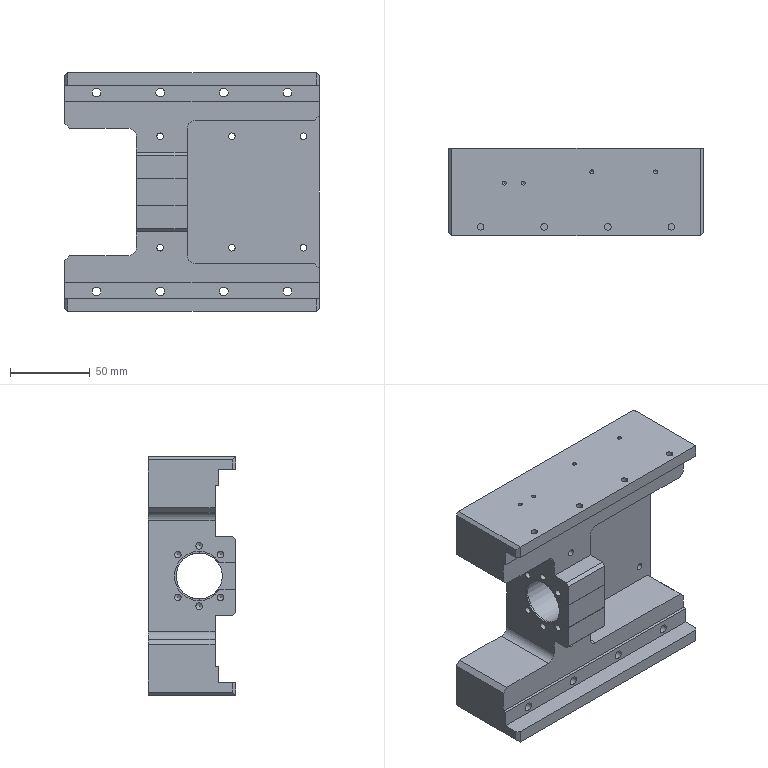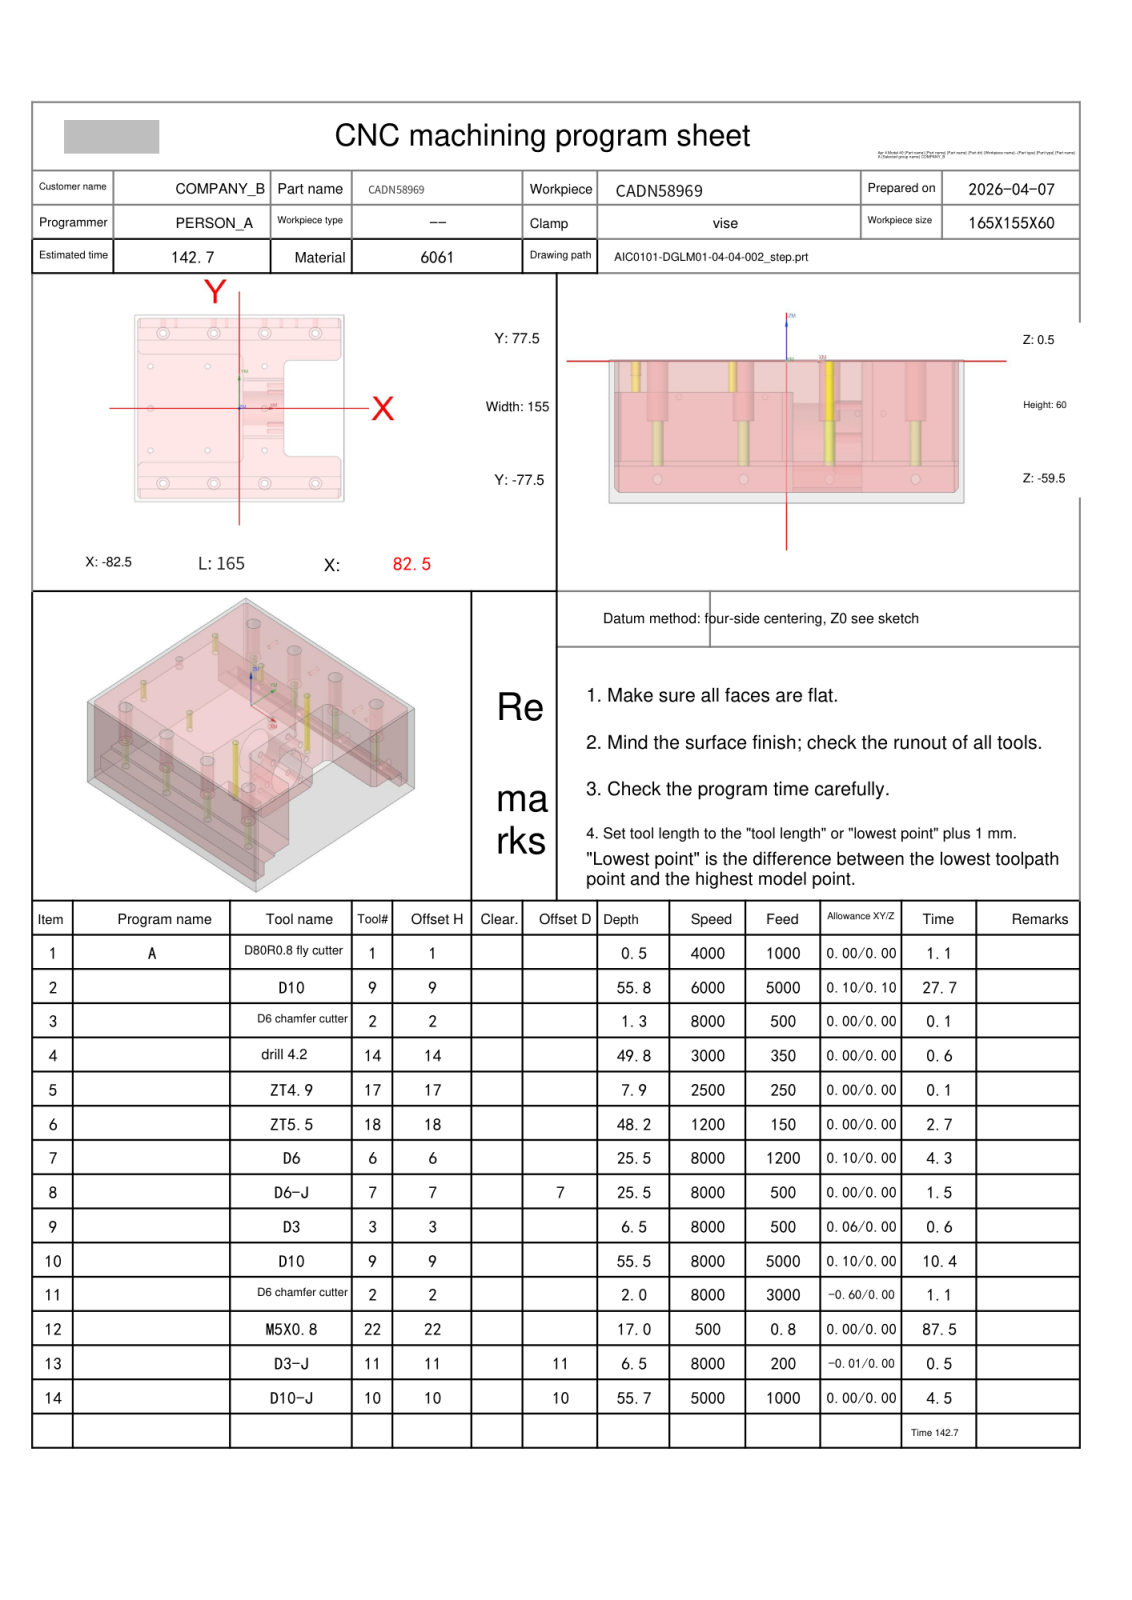NC program | NX | posted by the shop | part box 160 x 55 x 150 mm
Lines 12264 to 13088 of 15707:
N3 T02 M06
(D6 chamfer cutter D=6. R=0. H=02 ce=0.00 di=0.10)
G00 G90 G54 X60. Y-62.5 M03 S8000
G43 H02 Z20.
M08
G98 G81 X60. Y-62.5 Z-.8 R1. F500.
X20.
Y-35.
X-25.
X-20. Y-62.5
X-60.
X-70. Y-35.
Y0.0
Y35.
X-60. Y62.5
X-20.
X-25. Y35.
X20. Y0.0
Y35.
Y62.5
X60.
G80
G00 Z20.
G91 G28 Z0.0
M05
M09
G91 G28 Z0.0
M01
N4 T14 M06
(drill 4.2 D=4.2 DR_a=118 H=14)
G00 G90 G54 X-70. Y-35. M03 S3000
G43 H14 Z20.
M08
G98 G83 X-70. Y-35. Z-20.262 R1. F350. Q3.
X-25.
G98 G83 X20. Y-35. Z-49.262 R1. Q3.
Y35.
G98 G83 X-25. Y35. Z-20.262 R1. Q3.
X-70.
G80
G00 Z20.
G91 G28 Z0.0
M05
M09
G91 G28 Z0.0
M01
N5 T17 M06
(ZT4.9 D=4.9 DR_a=120 H=17)
G00 G90 G54 X20. Y0.0 M03 S2500
G43 H17 Z20.
M08
G98 G83 X20. Y0.0 Z-7.445 R1. F250. Q2.
X-70.
G80
G00 Z20.
G91 G28 Z0.0
M05
M09
G91 G28 Z0.0
M01
N6 T18 M06
(ZT5.5 D=5.5 DR_a=118 H=18)
G00 G90 G54 X60. Y62.5 M03 S1200
G43 H18 Z20.
M08
G98 G83 X60. Y62.5 Z-47.652 R1. F150. Q2.
X20.
X-20.
X-60.
Y-62.5
X-20.
X20.
X60.
G80
G00 Z20.
G91 G28 Z0.0
M05
M09
G91 G28 Z0.0
M01
N7 T06 M06
(D6  D=6. R=0. H=06 ce=0.10 di=0.00)
G00 G90 G54 X60. Y62.5 M03 S8000
G43 H06 Z20.
M08
Z.5
G03 X59.05 Y63.45 I-.95 J0.0 F1200.
X58.1 Y62.5 I0.0 J-.95
X58.1 Y62.5 Z0.0 I1.9 J0.0
X58.1 Y62.5 Z-.5 I1.9 J0.0
X58.1 Y62.5 Z-1. I1.9 J0.0
X58.1 Y62.5 Z-1.5 I1.9 J0.0
X58.1 Y62.5 Z-2. I1.9 J0.0
X58.1 Y62.5 Z-2.5 I1.9 J0.0
X58.1 Y62.5 Z-3. I1.9 J0.0
X58.1 Y62.5 Z-3.5 I1.9 J0.0
X58.1 Y62.5 Z-4. I1.9 J0.0
X58.1 Y62.5 Z-4.5 I1.9 J0.0
X58.1 Y62.5 Z-5. I1.9 J0.0
X58.1 Y62.5 Z-5.5 I1.9 J0.0
X58.1 Y62.5 Z-6. I1.9 J0.0
X58.1 Y62.5 Z-6.5 I1.9 J0.0
X58.1 Y62.5 Z-7. I1.9 J0.0
X58.1 Y62.5 Z-7.5 I1.9 J0.0
X58.1 Y62.5 Z-8. I1.9 J0.0
X58.1 Y62.5 Z-8.5 I1.9 J0.0
X58.1 Y62.5 Z-9. I1.9 J0.0
X58.1 Y62.5 Z-9.5 I1.9 J0.0
X58.1 Y62.5 Z-10. I1.9 J0.0
X58.1 Y62.5 Z-10.5 I1.9 J0.0
X58.1 Y62.5 Z-11. I1.9 J0.0
X58.1 Y62.5 Z-11.5 I1.9 J0.0
X58.1 Y62.5 Z-12. I1.9 J0.0
X58.1 Y62.5 Z-12.5 I1.9 J0.0
X58.1 Y62.5 Z-13. I1.9 J0.0
X58.1 Y62.5 Z-13.5 I1.9 J0.0
X58.1 Y62.5 Z-14. I1.9 J0.0
X58.1 Y62.5 Z-14.5 I1.9 J0.0
X58.1 Y62.5 Z-15. I1.9 J0.0
X58.1 Y62.5 Z-15.5 I1.9 J0.0
X58.1 Y62.5 Z-16. I1.9 J0.0
X58.1 Y62.5 Z-16.5 I1.9 J0.0
X58.1 Y62.5 Z-17. I1.9 J0.0
X58.1 Y62.5 Z-17.5 I1.9 J0.0
X58.1 Y62.5 Z-18. I1.9 J0.0
X58.1 Y62.5 Z-18.5 I1.9 J0.0
X58.1 Y62.5 Z-19. I1.9 J0.0
X58.1 Y62.5 Z-19.5 I1.9 J0.0
X58.1 Y62.5 Z-20. I1.9 J0.0
X58.1 Y62.5 Z-20.5 I1.9 J0.0
X58.1 Y62.5 Z-21. I1.9 J0.0
X58.1 Y62.5 Z-21.5 I1.9 J0.0
X58.1 Y62.5 Z-22. I1.9 J0.0
X58.1 Y62.5 Z-22.5 I1.9 J0.0
X58.1 Y62.5 Z-23. I1.9 J0.0
X58.1 Y62.5 Z-23.5 I1.9 J0.0
X58.1 Y62.5 Z-24. I1.9 J0.0
X58.1 Y62.5 Z-24.5 I1.9 J0.0
X58.1 Y62.5 Z-25. I1.9 J0.0
X60. Y60.6 I1.9 J0.0
X61.9 Y62.5 I0.0 J1.9
X60. Y64.4 I-1.9 J0.0
X58.1 Y62.5 I0.0 J-1.9
X59.05 Y61.55 I.95 J0.0
X60. Y62.5 I0.0 J.95
G00 Z20.
X20.
Z.5
G03 X19.05 Y63.45 I-.95 J0.0
X18.1 Y62.5 I0.0 J-.95
X18.1 Y62.5 Z0.0 I1.9 J0.0
X18.1 Y62.5 Z-.5 I1.9 J0.0
X18.1 Y62.5 Z-1. I1.9 J0.0
X18.1 Y62.5 Z-1.5 I1.9 J0.0
X18.1 Y62.5 Z-2. I1.9 J0.0
X18.1 Y62.5 Z-2.5 I1.9 J0.0
X18.1 Y62.5 Z-3. I1.9 J0.0
X18.1 Y62.5 Z-3.5 I1.9 J0.0
X18.1 Y62.5 Z-4. I1.9 J0.0
X18.1 Y62.5 Z-4.5 I1.9 J0.0
X18.1 Y62.5 Z-5. I1.9 J0.0
X18.1 Y62.5 Z-5.5 I1.9 J0.0
X18.1 Y62.5 Z-6. I1.9 J0.0
X18.1 Y62.5 Z-6.5 I1.9 J0.0
X18.1 Y62.5 Z-7. I1.9 J0.0
X18.1 Y62.5 Z-7.5 I1.9 J0.0
X18.1 Y62.5 Z-8. I1.9 J0.0
X18.1 Y62.5 Z-8.5 I1.9 J0.0
X18.1 Y62.5 Z-9. I1.9 J0.0
X18.1 Y62.5 Z-9.5 I1.9 J0.0
X18.1 Y62.5 Z-10. I1.9 J0.0
X18.1 Y62.5 Z-10.5 I1.9 J0.0
X18.1 Y62.5 Z-11. I1.9 J0.0
X18.1 Y62.5 Z-11.5 I1.9 J0.0
X18.1 Y62.5 Z-12. I1.9 J0.0
X18.1 Y62.5 Z-12.5 I1.9 J0.0
X18.1 Y62.5 Z-13. I1.9 J0.0
X18.1 Y62.5 Z-13.5 I1.9 J0.0
X18.1 Y62.5 Z-14. I1.9 J0.0
X18.1 Y62.5 Z-14.5 I1.9 J0.0
X18.1 Y62.5 Z-15. I1.9 J0.0
X18.1 Y62.5 Z-15.5 I1.9 J0.0
X18.1 Y62.5 Z-16. I1.9 J0.0
X18.1 Y62.5 Z-16.5 I1.9 J0.0
X18.1 Y62.5 Z-17. I1.9 J0.0
X18.1 Y62.5 Z-17.5 I1.9 J0.0
X18.1 Y62.5 Z-18. I1.9 J0.0
X18.1 Y62.5 Z-18.5 I1.9 J0.0
X18.1 Y62.5 Z-19. I1.9 J0.0
X18.1 Y62.5 Z-19.5 I1.9 J0.0
X18.1 Y62.5 Z-20. I1.9 J0.0
X18.1 Y62.5 Z-20.5 I1.9 J0.0
X18.1 Y62.5 Z-21. I1.9 J0.0
X18.1 Y62.5 Z-21.5 I1.9 J0.0
X18.1 Y62.5 Z-22. I1.9 J0.0
X18.1 Y62.5 Z-22.5 I1.9 J0.0
X18.1 Y62.5 Z-23. I1.9 J0.0
X18.1 Y62.5 Z-23.5 I1.9 J0.0
X18.1 Y62.5 Z-24. I1.9 J0.0
X18.1 Y62.5 Z-24.5 I1.9 J0.0
X18.1 Y62.5 Z-25. I1.9 J0.0
X20. Y60.6 I1.9 J0.0
X21.9 Y62.5 I0.0 J1.9
X20. Y64.4 I-1.9 J0.0
X18.1 Y62.5 I0.0 J-1.9
X19.05 Y61.55 I.95 J0.0
X20. Y62.5 I0.0 J.95
G00 Z20.
X-20.
Z.5
G03 X-20.95 Y63.45 I-.95 J0.0
X-21.9 Y62.5 I0.0 J-.95
X-21.9 Y62.5 Z0.0 I1.9 J0.0
X-21.9 Y62.5 Z-.5 I1.9 J0.0
X-21.9 Y62.5 Z-1. I1.9 J0.0
X-21.9 Y62.5 Z-1.5 I1.9 J0.0
X-21.9 Y62.5 Z-2. I1.9 J0.0
X-21.9 Y62.5 Z-2.5 I1.9 J0.0
X-21.9 Y62.5 Z-3. I1.9 J0.0
X-21.9 Y62.5 Z-3.5 I1.9 J0.0
X-21.9 Y62.5 Z-4. I1.9 J0.0
X-21.9 Y62.5 Z-4.5 I1.9 J0.0
X-21.9 Y62.5 Z-5. I1.9 J0.0
X-21.9 Y62.5 Z-5.5 I1.9 J0.0
X-21.9 Y62.5 Z-6. I1.9 J0.0
X-21.9 Y62.5 Z-6.5 I1.9 J0.0
X-21.9 Y62.5 Z-7. I1.9 J0.0
X-21.9 Y62.5 Z-7.5 I1.9 J0.0
X-21.9 Y62.5 Z-8. I1.9 J0.0
X-21.9 Y62.5 Z-8.5 I1.9 J0.0
X-21.9 Y62.5 Z-9. I1.9 J0.0
X-21.9 Y62.5 Z-9.5 I1.9 J0.0
X-21.9 Y62.5 Z-10. I1.9 J0.0
X-21.9 Y62.5 Z-10.5 I1.9 J0.0
X-21.9 Y62.5 Z-11. I1.9 J0.0
X-21.9 Y62.5 Z-11.5 I1.9 J0.0
X-21.9 Y62.5 Z-12. I1.9 J0.0
X-21.9 Y62.5 Z-12.5 I1.9 J0.0
X-21.9 Y62.5 Z-13. I1.9 J0.0
X-21.9 Y62.5 Z-13.5 I1.9 J0.0
X-21.9 Y62.5 Z-14. I1.9 J0.0
X-21.9 Y62.5 Z-14.5 I1.9 J0.0
X-21.9 Y62.5 Z-15. I1.9 J0.0
X-21.9 Y62.5 Z-15.5 I1.9 J0.0
X-21.9 Y62.5 Z-16. I1.9 J0.0
X-21.9 Y62.5 Z-16.5 I1.9 J0.0
X-21.9 Y62.5 Z-17. I1.9 J0.0
X-21.9 Y62.5 Z-17.5 I1.9 J0.0
X-21.9 Y62.5 Z-18. I1.9 J0.0
X-21.9 Y62.5 Z-18.5 I1.9 J0.0
X-21.9 Y62.5 Z-19. I1.9 J0.0
X-21.9 Y62.5 Z-19.5 I1.9 J0.0
X-21.9 Y62.5 Z-20. I1.9 J0.0
X-21.9 Y62.5 Z-20.5 I1.9 J0.0
X-21.9 Y62.5 Z-21. I1.9 J0.0
X-21.9 Y62.5 Z-21.5 I1.9 J0.0
X-21.9 Y62.5 Z-22. I1.9 J0.0
X-21.9 Y62.5 Z-22.5 I1.9 J0.0
X-21.9 Y62.5 Z-23. I1.9 J0.0
X-21.9 Y62.5 Z-23.5 I1.9 J0.0
X-21.9 Y62.5 Z-24. I1.9 J0.0
X-21.9 Y62.5 Z-24.5 I1.9 J0.0
X-21.9 Y62.5 Z-25. I1.9 J0.0
X-20. Y60.6 I1.9 J0.0
X-18.1 Y62.5 I0.0 J1.9
X-20. Y64.4 I-1.9 J0.0
X-21.9 Y62.5 I0.0 J-1.9
X-20.95 Y61.55 I.95 J0.0
X-20. Y62.5 I0.0 J.95
G00 Z20.
X-60.
Z.5
G03 X-60.95 Y63.45 I-.95 J0.0
X-61.9 Y62.5 I0.0 J-.95
X-61.9 Y62.5 Z0.0 I1.9 J0.0
X-61.9 Y62.5 Z-.5 I1.9 J0.0
X-61.9 Y62.5 Z-1. I1.9 J0.0
X-61.9 Y62.5 Z-1.5 I1.9 J0.0
X-61.9 Y62.5 Z-2. I1.9 J0.0
X-61.9 Y62.5 Z-2.5 I1.9 J0.0
X-61.9 Y62.5 Z-3. I1.9 J0.0
X-61.9 Y62.5 Z-3.5 I1.9 J0.0
X-61.9 Y62.5 Z-4. I1.9 J0.0
X-61.9 Y62.5 Z-4.5 I1.9 J0.0
X-61.9 Y62.5 Z-5. I1.9 J0.0
X-61.9 Y62.5 Z-5.5 I1.9 J0.0
X-61.9 Y62.5 Z-6. I1.9 J0.0
X-61.9 Y62.5 Z-6.5 I1.9 J0.0
X-61.9 Y62.5 Z-7. I1.9 J0.0
X-61.9 Y62.5 Z-7.5 I1.9 J0.0
X-61.9 Y62.5 Z-8. I1.9 J0.0
X-61.9 Y62.5 Z-8.5 I1.9 J0.0
X-61.9 Y62.5 Z-9. I1.9 J0.0
X-61.9 Y62.5 Z-9.5 I1.9 J0.0
X-61.9 Y62.5 Z-10. I1.9 J0.0
X-61.9 Y62.5 Z-10.5 I1.9 J0.0
X-61.9 Y62.5 Z-11. I1.9 J0.0
X-61.9 Y62.5 Z-11.5 I1.9 J0.0
X-61.9 Y62.5 Z-12. I1.9 J0.0
X-61.9 Y62.5 Z-12.5 I1.9 J0.0
X-61.9 Y62.5 Z-13. I1.9 J0.0
X-61.9 Y62.5 Z-13.5 I1.9 J0.0
X-61.9 Y62.5 Z-14. I1.9 J0.0
X-61.9 Y62.5 Z-14.5 I1.9 J0.0
X-61.9 Y62.5 Z-15. I1.9 J0.0
X-61.9 Y62.5 Z-15.5 I1.9 J0.0
X-61.9 Y62.5 Z-16. I1.9 J0.0
X-61.9 Y62.5 Z-16.5 I1.9 J0.0
X-61.9 Y62.5 Z-17. I1.9 J0.0
X-61.9 Y62.5 Z-17.5 I1.9 J0.0
X-61.9 Y62.5 Z-18. I1.9 J0.0
X-61.9 Y62.5 Z-18.5 I1.9 J0.0
X-61.9 Y62.5 Z-19. I1.9 J0.0
X-61.9 Y62.5 Z-19.5 I1.9 J0.0
X-61.9 Y62.5 Z-20. I1.9 J0.0
X-61.9 Y62.5 Z-20.5 I1.9 J0.0
X-61.9 Y62.5 Z-21. I1.9 J0.0
X-61.9 Y62.5 Z-21.5 I1.9 J0.0
X-61.9 Y62.5 Z-22. I1.9 J0.0
X-61.9 Y62.5 Z-22.5 I1.9 J0.0
X-61.9 Y62.5 Z-23. I1.9 J0.0
X-61.9 Y62.5 Z-23.5 I1.9 J0.0
X-61.9 Y62.5 Z-24. I1.9 J0.0
X-61.9 Y62.5 Z-24.5 I1.9 J0.0
X-61.9 Y62.5 Z-25. I1.9 J0.0
X-60. Y60.6 I1.9 J0.0
X-58.1 Y62.5 I0.0 J1.9
X-60. Y64.4 I-1.9 J0.0
X-61.9 Y62.5 I0.0 J-1.9
X-60.95 Y61.55 I.95 J0.0
X-60. Y62.5 I0.0 J.95
G00 Z20.
Y-62.5
Z.5
G03 X-60.95 Y-61.55 I-.95 J0.0
X-61.9 Y-62.5 I0.0 J-.95
X-61.9 Y-62.5 Z0.0 I1.9 J0.0
X-61.9 Y-62.5 Z-.5 I1.9 J0.0
X-61.9 Y-62.5 Z-1. I1.9 J0.0
X-61.9 Y-62.5 Z-1.5 I1.9 J0.0
X-61.9 Y-62.5 Z-2. I1.9 J0.0
X-61.9 Y-62.5 Z-2.5 I1.9 J0.0
X-61.9 Y-62.5 Z-3. I1.9 J0.0
X-61.9 Y-62.5 Z-3.5 I1.9 J0.0
X-61.9 Y-62.5 Z-4. I1.9 J0.0
X-61.9 Y-62.5 Z-4.5 I1.9 J0.0
X-61.9 Y-62.5 Z-5. I1.9 J0.0
X-61.9 Y-62.5 Z-5.5 I1.9 J0.0
X-61.9 Y-62.5 Z-6. I1.9 J0.0
X-61.9 Y-62.5 Z-6.5 I1.9 J0.0
X-61.9 Y-62.5 Z-7. I1.9 J0.0
X-61.9 Y-62.5 Z-7.5 I1.9 J0.0
X-61.9 Y-62.5 Z-8. I1.9 J0.0
X-61.9 Y-62.5 Z-8.5 I1.9 J0.0
X-61.9 Y-62.5 Z-9. I1.9 J0.0
X-61.9 Y-62.5 Z-9.5 I1.9 J0.0
X-61.9 Y-62.5 Z-10. I1.9 J0.0
X-61.9 Y-62.5 Z-10.5 I1.9 J0.0
X-61.9 Y-62.5 Z-11. I1.9 J0.0
X-61.9 Y-62.5 Z-11.5 I1.9 J0.0
X-61.9 Y-62.5 Z-12. I1.9 J0.0
X-61.9 Y-62.5 Z-12.5 I1.9 J0.0
X-61.9 Y-62.5 Z-13. I1.9 J0.0
X-61.9 Y-62.5 Z-13.5 I1.9 J0.0
X-61.9 Y-62.5 Z-14. I1.9 J0.0
X-61.9 Y-62.5 Z-14.5 I1.9 J0.0
X-61.9 Y-62.5 Z-15. I1.9 J0.0
X-61.9 Y-62.5 Z-15.5 I1.9 J0.0
X-61.9 Y-62.5 Z-16. I1.9 J0.0
X-61.9 Y-62.5 Z-16.5 I1.9 J0.0
X-61.9 Y-62.5 Z-17. I1.9 J0.0
X-61.9 Y-62.5 Z-17.5 I1.9 J0.0
X-61.9 Y-62.5 Z-18. I1.9 J0.0
X-61.9 Y-62.5 Z-18.5 I1.9 J0.0
X-61.9 Y-62.5 Z-19. I1.9 J0.0
X-61.9 Y-62.5 Z-19.5 I1.9 J0.0
X-61.9 Y-62.5 Z-20. I1.9 J0.0
X-61.9 Y-62.5 Z-20.5 I1.9 J0.0
X-61.9 Y-62.5 Z-21. I1.9 J0.0
X-61.9 Y-62.5 Z-21.5 I1.9 J0.0
X-61.9 Y-62.5 Z-22. I1.9 J0.0
X-61.9 Y-62.5 Z-22.5 I1.9 J0.0
X-61.9 Y-62.5 Z-23. I1.9 J0.0
X-61.9 Y-62.5 Z-23.5 I1.9 J0.0
X-61.9 Y-62.5 Z-24. I1.9 J0.0
X-61.9 Y-62.5 Z-24.5 I1.9 J0.0
X-61.9 Y-62.5 Z-25. I1.9 J0.0
X-60. Y-64.4 I1.9 J0.0
X-58.1 Y-62.5 I0.0 J1.9
X-60. Y-60.6 I-1.9 J0.0
X-61.9 Y-62.5 I0.0 J-1.9
X-60.95 Y-63.45 I.95 J0.0
X-60. Y-62.5 I0.0 J.95
G00 Z20.
X-20.
Z.5
G03 X-20.95 Y-61.55 I-.95 J0.0
X-21.9 Y-62.5 I0.0 J-.95
X-21.9 Y-62.5 Z0.0 I1.9 J0.0
X-21.9 Y-62.5 Z-.5 I1.9 J0.0
X-21.9 Y-62.5 Z-1. I1.9 J0.0
X-21.9 Y-62.5 Z-1.5 I1.9 J0.0
X-21.9 Y-62.5 Z-2. I1.9 J0.0
X-21.9 Y-62.5 Z-2.5 I1.9 J0.0
X-21.9 Y-62.5 Z-3. I1.9 J0.0
X-21.9 Y-62.5 Z-3.5 I1.9 J0.0
X-21.9 Y-62.5 Z-4. I1.9 J0.0
X-21.9 Y-62.5 Z-4.5 I1.9 J0.0
X-21.9 Y-62.5 Z-5. I1.9 J0.0
X-21.9 Y-62.5 Z-5.5 I1.9 J0.0
X-21.9 Y-62.5 Z-6. I1.9 J0.0
X-21.9 Y-62.5 Z-6.5 I1.9 J0.0
X-21.9 Y-62.5 Z-7. I1.9 J0.0
X-21.9 Y-62.5 Z-7.5 I1.9 J0.0
X-21.9 Y-62.5 Z-8. I1.9 J0.0
X-21.9 Y-62.5 Z-8.5 I1.9 J0.0
X-21.9 Y-62.5 Z-9. I1.9 J0.0
X-21.9 Y-62.5 Z-9.5 I1.9 J0.0
X-21.9 Y-62.5 Z-10. I1.9 J0.0
X-21.9 Y-62.5 Z-10.5 I1.9 J0.0
X-21.9 Y-62.5 Z-11. I1.9 J0.0
X-21.9 Y-62.5 Z-11.5 I1.9 J0.0
X-21.9 Y-62.5 Z-12. I1.9 J0.0
X-21.9 Y-62.5 Z-12.5 I1.9 J0.0
X-21.9 Y-62.5 Z-13. I1.9 J0.0
X-21.9 Y-62.5 Z-13.5 I1.9 J0.0
X-21.9 Y-62.5 Z-14. I1.9 J0.0
X-21.9 Y-62.5 Z-14.5 I1.9 J0.0
X-21.9 Y-62.5 Z-15. I1.9 J0.0
X-21.9 Y-62.5 Z-15.5 I1.9 J0.0
X-21.9 Y-62.5 Z-16. I1.9 J0.0
X-21.9 Y-62.5 Z-16.5 I1.9 J0.0
X-21.9 Y-62.5 Z-17. I1.9 J0.0
X-21.9 Y-62.5 Z-17.5 I1.9 J0.0
X-21.9 Y-62.5 Z-18. I1.9 J0.0
X-21.9 Y-62.5 Z-18.5 I1.9 J0.0
X-21.9 Y-62.5 Z-19. I1.9 J0.0
X-21.9 Y-62.5 Z-19.5 I1.9 J0.0
X-21.9 Y-62.5 Z-20. I1.9 J0.0
X-21.9 Y-62.5 Z-20.5 I1.9 J0.0
X-21.9 Y-62.5 Z-21. I1.9 J0.0
X-21.9 Y-62.5 Z-21.5 I1.9 J0.0
X-21.9 Y-62.5 Z-22. I1.9 J0.0
X-21.9 Y-62.5 Z-22.5 I1.9 J0.0
X-21.9 Y-62.5 Z-23. I1.9 J0.0
X-21.9 Y-62.5 Z-23.5 I1.9 J0.0
X-21.9 Y-62.5 Z-24. I1.9 J0.0
X-21.9 Y-62.5 Z-24.5 I1.9 J0.0
X-21.9 Y-62.5 Z-25. I1.9 J0.0
X-20. Y-64.4 I1.9 J0.0
X-18.1 Y-62.5 I0.0 J1.9
X-20. Y-60.6 I-1.9 J0.0
X-21.9 Y-62.5 I0.0 J-1.9
X-20.95 Y-63.45 I.95 J0.0
X-20. Y-62.5 I0.0 J.95
G00 Z20.
X20.
Z.5
G03 X19.05 Y-61.55 I-.95 J0.0
X18.1 Y-62.5 I0.0 J-.95
X18.1 Y-62.5 Z0.0 I1.9 J0.0
X18.1 Y-62.5 Z-.5 I1.9 J0.0
X18.1 Y-62.5 Z-1. I1.9 J0.0
X18.1 Y-62.5 Z-1.5 I1.9 J0.0
X18.1 Y-62.5 Z-2. I1.9 J0.0
X18.1 Y-62.5 Z-2.5 I1.9 J0.0
X18.1 Y-62.5 Z-3. I1.9 J0.0
X18.1 Y-62.5 Z-3.5 I1.9 J0.0
X18.1 Y-62.5 Z-4. I1.9 J0.0
X18.1 Y-62.5 Z-4.5 I1.9 J0.0
X18.1 Y-62.5 Z-5. I1.9 J0.0
X18.1 Y-62.5 Z-5.5 I1.9 J0.0
X18.1 Y-62.5 Z-6. I1.9 J0.0
X18.1 Y-62.5 Z-6.5 I1.9 J0.0
X18.1 Y-62.5 Z-7. I1.9 J0.0
X18.1 Y-62.5 Z-7.5 I1.9 J0.0
X18.1 Y-62.5 Z-8. I1.9 J0.0
X18.1 Y-62.5 Z-8.5 I1.9 J0.0
X18.1 Y-62.5 Z-9. I1.9 J0.0
X18.1 Y-62.5 Z-9.5 I1.9 J0.0
X18.1 Y-62.5 Z-10. I1.9 J0.0
X18.1 Y-62.5 Z-10.5 I1.9 J0.0
X18.1 Y-62.5 Z-11. I1.9 J0.0
X18.1 Y-62.5 Z-11.5 I1.9 J0.0
X18.1 Y-62.5 Z-12. I1.9 J0.0
X18.1 Y-62.5 Z-12.5 I1.9 J0.0
X18.1 Y-62.5 Z-13. I1.9 J0.0
X18.1 Y-62.5 Z-13.5 I1.9 J0.0
X18.1 Y-62.5 Z-14. I1.9 J0.0
X18.1 Y-62.5 Z-14.5 I1.9 J0.0
X18.1 Y-62.5 Z-15. I1.9 J0.0
X18.1 Y-62.5 Z-15.5 I1.9 J0.0
X18.1 Y-62.5 Z-16. I1.9 J0.0
X18.1 Y-62.5 Z-16.5 I1.9 J0.0
X18.1 Y-62.5 Z-17. I1.9 J0.0
X18.1 Y-62.5 Z-17.5 I1.9 J0.0
X18.1 Y-62.5 Z-18. I1.9 J0.0
X18.1 Y-62.5 Z-18.5 I1.9 J0.0
X18.1 Y-62.5 Z-19. I1.9 J0.0
X18.1 Y-62.5 Z-19.5 I1.9 J0.0
X18.1 Y-62.5 Z-20. I1.9 J0.0
X18.1 Y-62.5 Z-20.5 I1.9 J0.0
X18.1 Y-62.5 Z-21. I1.9 J0.0
X18.1 Y-62.5 Z-21.5 I1.9 J0.0
X18.1 Y-62.5 Z-22. I1.9 J0.0
X18.1 Y-62.5 Z-22.5 I1.9 J0.0
X18.1 Y-62.5 Z-23. I1.9 J0.0
X18.1 Y-62.5 Z-23.5 I1.9 J0.0
X18.1 Y-62.5 Z-24. I1.9 J0.0
X18.1 Y-62.5 Z-24.5 I1.9 J0.0
X18.1 Y-62.5 Z-25. I1.9 J0.0
X20. Y-64.4 I1.9 J0.0
X21.9 Y-62.5 I0.0 J1.9
X20. Y-60.6 I-1.9 J0.0
X18.1 Y-62.5 I0.0 J-1.9
X19.05 Y-63.45 I.95 J0.0
X20. Y-62.5 I0.0 J.95
G00 Z20.
X60.
Z.5
G03 X59.05 Y-61.55 I-.95 J0.0
X58.1 Y-62.5 I0.0 J-.95
X58.1 Y-62.5 Z0.0 I1.9 J0.0
X58.1 Y-62.5 Z-.5 I1.9 J0.0
X58.1 Y-62.5 Z-1. I1.9 J0.0
X58.1 Y-62.5 Z-1.5 I1.9 J0.0
X58.1 Y-62.5 Z-2. I1.9 J0.0
X58.1 Y-62.5 Z-2.5 I1.9 J0.0
X58.1 Y-62.5 Z-3. I1.9 J0.0
X58.1 Y-62.5 Z-3.5 I1.9 J0.0
X58.1 Y-62.5 Z-4. I1.9 J0.0
X58.1 Y-62.5 Z-4.5 I1.9 J0.0
X58.1 Y-62.5 Z-5. I1.9 J0.0
X58.1 Y-62.5 Z-5.5 I1.9 J0.0
X58.1 Y-62.5 Z-6. I1.9 J0.0
X58.1 Y-62.5 Z-6.5 I1.9 J0.0
X58.1 Y-62.5 Z-7. I1.9 J0.0
X58.1 Y-62.5 Z-7.5 I1.9 J0.0
X58.1 Y-62.5 Z-8. I1.9 J0.0
X58.1 Y-62.5 Z-8.5 I1.9 J0.0
X58.1 Y-62.5 Z-9. I1.9 J0.0
X58.1 Y-62.5 Z-9.5 I1.9 J0.0
X58.1 Y-62.5 Z-10. I1.9 J0.0
X58.1 Y-62.5 Z-10.5 I1.9 J0.0
X58.1 Y-62.5 Z-11. I1.9 J0.0
X58.1 Y-62.5 Z-11.5 I1.9 J0.0
X58.1 Y-62.5 Z-12. I1.9 J0.0
X58.1 Y-62.5 Z-12.5 I1.9 J0.0
X58.1 Y-62.5 Z-13. I1.9 J0.0
X58.1 Y-62.5 Z-13.5 I1.9 J0.0
X58.1 Y-62.5 Z-14. I1.9 J0.0
X58.1 Y-62.5 Z-14.5 I1.9 J0.0
X58.1 Y-62.5 Z-15. I1.9 J0.0
X58.1 Y-62.5 Z-15.5 I1.9 J0.0
X58.1 Y-62.5 Z-16. I1.9 J0.0
X58.1 Y-62.5 Z-16.5 I1.9 J0.0
X58.1 Y-62.5 Z-17. I1.9 J0.0
X58.1 Y-62.5 Z-17.5 I1.9 J0.0
X58.1 Y-62.5 Z-18. I1.9 J0.0
X58.1 Y-62.5 Z-18.5 I1.9 J0.0
X58.1 Y-62.5 Z-19. I1.9 J0.0
X58.1 Y-62.5 Z-19.5 I1.9 J0.0
X58.1 Y-62.5 Z-20. I1.9 J0.0
X58.1 Y-62.5 Z-20.5 I1.9 J0.0
X58.1 Y-62.5 Z-21. I1.9 J0.0
X58.1 Y-62.5 Z-21.5 I1.9 J0.0
X58.1 Y-62.5 Z-22. I1.9 J0.0
X58.1 Y-62.5 Z-22.5 I1.9 J0.0
X58.1 Y-62.5 Z-23. I1.9 J0.0
X58.1 Y-62.5 Z-23.5 I1.9 J0.0
X58.1 Y-62.5 Z-24. I1.9 J0.0
X58.1 Y-62.5 Z-24.5 I1.9 J0.0
X58.1 Y-62.5 Z-25. I1.9 J0.0
X60. Y-64.4 I1.9 J0.0
X61.9 Y-62.5 I0.0 J1.9
X60. Y-60.6 I-1.9 J0.0
X58.1 Y-62.5 I0.0 J-1.9
X59.05 Y-63.45 I.95 J0.0
X60. Y-62.5 I0.0 J.95
G00 Z20.
G91 G28 Z0.0
M05
M09
G91 G28 Z0.0
M01
N8 T07 M06
(D6-J  D=6. R=0. H=07 ce=0.00 di=0.00)
G00 G90 G54 X60. Y62.5 M03 S8000
G43 H07 Z20.
M08
Z0.0
G41 D07
G01 X59.96 Y62.696 F500.
G03 X58.99 Y63.49 I-.97 J-.196
X58. Y62.5 I0.0 J-.99
X58. Y62.5 Z-5. I2. J0.0
X58. Y62.5 Z-10. I2. J0.0
X58. Y62.5 Z-15. I2. J0.0
X58. Y62.5 Z-20. I2. J0.0
X58. Y62.5 Z-25. I2. J0.0
X60. Y60.5 I2. J0.0
X62. Y62.5 I0.0 J2.
X60. Y64.5 I-2. J0.0
X58. Y62.5 I0.0 J-2.
X58.99 Y61.51 I.99 J0.0
X59.96 Y62.304 I0.0 J.99
G01 G40 X60. Y62.5
G00 Z20.
X20.
Z0.0
G41 D07
G01 X19.96 Y62.696
G03 X18.99 Y63.49 I-.97 J-.196
X18. Y62.5 I0.0 J-.99
X18. Y62.5 Z-5. I2. J0.0
X18. Y62.5 Z-10. I2. J0.0
X18. Y62.5 Z-15. I2. J0.0
X18. Y62.5 Z-20. I2. J0.0
X18. Y62.5 Z-25. I2. J0.0
X20. Y60.5 I2. J0.0
X22. Y62.5 I0.0 J2.
X20. Y64.5 I-2. J0.0
X18. Y62.5 I0.0 J-2.
X18.99 Y61.51 I.99 J0.0
X19.96 Y62.304 I0.0 J.99
G01 G40 X20. Y62.5
G00 Z20.
X-20.
Z0.0
G41 D07
G01 X-20.04 Y62.696
G03 X-21.01 Y63.49 I-.97 J-.196
X-22. Y62.5 I0.0 J-.99
X-22. Y62.5 Z-5. I2. J0.0
X-22. Y62.5 Z-10. I2. J0.0
X-22. Y62.5 Z-15. I2. J0.0
X-22. Y62.5 Z-20. I2. J0.0
X-22. Y62.5 Z-25. I2. J0.0
X-20. Y60.5 I2. J0.0
X-18. Y62.5 I0.0 J2.
X-20. Y64.5 I-2. J0.0
X-22. Y62.5 I0.0 J-2.
X-21.01 Y61.51 I.99 J0.0
X-20.04 Y62.304 I0.0 J.99
G01 G40 X-20. Y62.5
G00 Z20.
X-60.
Z0.0
G41 D07
G01 X-60.04 Y62.696
G03 X-61.01 Y63.49 I-.97 J-.196
X-62. Y62.5 I0.0 J-.99
X-62. Y62.5 Z-5. I2. J0.0
X-62. Y62.5 Z-10. I2. J0.0
X-62. Y62.5 Z-15. I2. J0.0
X-62. Y62.5 Z-20. I2. J0.0
X-62. Y62.5 Z-25. I2. J0.0
X-60. Y60.5 I2. J0.0
X-58. Y62.5 I0.0 J2.
X-60. Y64.5 I-2. J0.0
X-62. Y62.5 I0.0 J-2.
X-61.01 Y61.51 I.99 J0.0
X-60.04 Y62.304 I0.0 J.99
G01 G40 X-60. Y62.5
G00 Z20.
Y-62.5
Z0.0
G41 D07
G01 X-60.04 Y-62.304
G03 X-61.01 Y-61.51 I-.97 J-.196
X-62. Y-62.5 I0.0 J-.99
X-62. Y-62.5 Z-5. I2. J0.0
X-62. Y-62.5 Z-10. I2. J0.0
X-62. Y-62.5 Z-15. I2. J0.0
X-62. Y-62.5 Z-20. I2. J0.0
X-62. Y-62.5 Z-25. I2. J0.0
X-60. Y-64.5 I2. J0.0
X-58. Y-62.5 I0.0 J2.
X-60. Y-60.5 I-2. J0.0
X-62. Y-62.5 I0.0 J-2.
X-61.01 Y-63.49 I.99 J0.0
X-60.04 Y-62.696 I0.0 J.99
G01 G40 X-60. Y-62.5
G00 Z20.
X-20.
Z0.0
G41 D07
G01 X-20.04 Y-62.304
G03 X-21.01 Y-61.51 I-.97 J-.196
X-22. Y-62.5 I0.0 J-.99
X-22. Y-62.5 Z-5. I2. J0.0
X-22. Y-62.5 Z-10. I2. J0.0
X-22. Y-62.5 Z-15. I2. J0.0
X-22. Y-62.5 Z-20. I2. J0.0
X-22. Y-62.5 Z-25. I2. J0.0
X-20. Y-64.5 I2. J0.0
X-18. Y-62.5 I0.0 J2.
X-20. Y-60.5 I-2. J0.0
X-22. Y-62.5 I0.0 J-2.
X-21.01 Y-63.49 I.99 J0.0
X-20.04 Y-62.696 I0.0 J.99
G01 G40 X-20. Y-62.5
G00 Z20.
X20.
Z0.0
G41 D07
G01 X19.96 Y-62.304
G03 X18.99 Y-61.51 I-.97 J-.196
X18. Y-62.5 I0.0 J-.99
X18. Y-62.5 Z-5. I2. J0.0
X18. Y-62.5 Z-10. I2. J0.0
X18. Y-62.5 Z-15. I2. J0.0
X18. Y-62.5 Z-20. I2. J0.0
X18. Y-62.5 Z-25. I2. J0.0
X20. Y-64.5 I2. J0.0
X22. Y-62.5 I0.0 J2.
X20. Y-60.5 I-2. J0.0
X18. Y-62.5 I0.0 J-2.
X18.99 Y-63.49 I.99 J0.0
X19.96 Y-62.696 I0.0 J.99
G01 G40 X20. Y-62.5
G00 Z20.
X60.
Z0.0
G41 D07
G01 X59.96 Y-62.304
G03 X58.99 Y-61.51 I-.97 J-.196
X58. Y-62.5 I0.0 J-.99
X58. Y-62.5 Z-5. I2. J0.0
X58. Y-62.5 Z-10. I2. J0.0
X58. Y-62.5 Z-15. I2. J0.0
X58. Y-62.5 Z-20. I2. J0.0
X58. Y-62.5 Z-25. I2. J0.0
X60. Y-64.5 I2. J0.0
X62. Y-62.5 I0.0 J2.
X60. Y-60.5 I-2. J0.0
X58. Y-62.5 I0.0 J-2.
X58.99 Y-63.49 I.99 J0.0
X59.96 Y-62.696 I0.0 J.99
G01 G40 X60. Y-62.5
G00 Z20.
G91 G28 Z0.0
M05
M09
G91 G28 Z0.0
M01
N9 T03 M06
(D3  D=3. R=0. H=03 ce=0.06 di=0.00)
G00 G90 G54 X20. Y0.0 M03 S8000
G43 H03 Z20.
M08
Z.5
G03 X19.53 Y.47 I-.47 J0.0 F500.
X19.06 Y0.0 I0.0 J-.47
X19.06 Y0.0 Z.2 I.94 J0.0
X19.06 Y0.0 Z-.1 I.94 J0.0
X19.06 Y0.0 Z-.4 I.94 J0.0
X19.06 Y0.0 Z-.7 I.94 J0.0
X19.06 Y0.0 Z-1. I.94 J0.0
X19.06 Y0.0 Z-1.3 I.94 J0.0
X19.06 Y0.0 Z-1.6 I.94 J0.0
X19.06 Y0.0 Z-1.9 I.94 J0.0
X19.06 Y0.0 Z-2.2 I.94 J0.0
X19.06 Y0.0 Z-2.5 I.94 J0.0
X19.06 Y0.0 Z-2.8 I.94 J0.0
X19.06 Y0.0 Z-3.1 I.94 J0.0
X19.06 Y0.0 Z-3.4 I.94 J0.0
X19.06 Y0.0 Z-3.7 I.94 J0.0
X19.06 Y0.0 Z-4. I.94 J0.0
X19.06 Y0.0 Z-4.3 I.94 J0.0
X19.06 Y0.0 Z-4.6 I.94 J0.0
X19.06 Y0.0 Z-4.9 I.94 J0.0
X19.06 Y0.0 Z-5.2 I.94 J0.0
X19.06 Y0.0 Z-5.5 I.94 J0.0
X19.06 Y0.0 Z-5.8 I.94 J0.0
X20.47 Y.814 Z-6. I.94 J0.0
X20. Y.94 I-.47 J-.814
X19.06 Y0.0 I0.0 J-.94
X20. Y-.94 I.94 J0.0
X20.94 Y0.0 I0.0 J.94
X20.47 Y.814 I-.94 J0.0
X20.235 Y.877 I-.235 J-.407
X19.765 Y.407 I0.0 J-.47
X20. Y0.0 I.47 J0.0
G00 Z20.
X-70.
Z.5
G03 X-70.47 Y.47 I-.47 J0.0
X-70.94 Y0.0 I0.0 J-.47
X-70.94 Y0.0 Z.2 I.94 J0.0
X-70.94 Y0.0 Z-.1 I.94 J0.0
X-70.94 Y0.0 Z-.4 I.94 J0.0
X-70.94 Y0.0 Z-.7 I.94 J0.0
X-70.94 Y0.0 Z-1. I.94 J0.0
X-70.94 Y0.0 Z-1.3 I.94 J0.0
X-70.94 Y0.0 Z-1.6 I.94 J0.0
X-70.94 Y0.0 Z-1.9 I.94 J0.0
X-70.94 Y0.0 Z-2.2 I.94 J0.0
X-70.94 Y0.0 Z-2.5 I.94 J0.0
X-70.94 Y0.0 Z-2.8 I.94 J0.0
X-70.94 Y0.0 Z-3.1 I.94 J0.0
X-70.94 Y0.0 Z-3.4 I.94 J0.0
X-70.94 Y0.0 Z-3.7 I.94 J0.0
X-70.94 Y0.0 Z-4. I.94 J0.0
X-70.94 Y0.0 Z-4.3 I.94 J0.0
X-70.94 Y0.0 Z-4.6 I.94 J0.0
X-70.94 Y0.0 Z-4.9 I.94 J0.0
X-70.94 Y0.0 Z-5.2 I.94 J0.0
X-70.94 Y0.0 Z-5.5 I.94 J0.0
X-70.94 Y0.0 Z-5.8 I.94 J0.0
X-69.53 Y.814 Z-6. I.94 J0.0
X-70. Y.94 I-.47 J-.814
X-70.94 Y0.0 I0.0 J-.94
X-70. Y-.94 I.94 J0.0
X-69.06 Y0.0 I0.0 J.94
X-69.53 Y.814 I-.94 J0.0
X-69.765 Y.877 I-.235 J-.407
X-70.235 Y.407 I0.0 J-.47
X-70. Y0.0 I.47 J0.0
G00 Z20.
G91 G28 Z0.0
M05
M09
G91 G28 Z0.0
M01